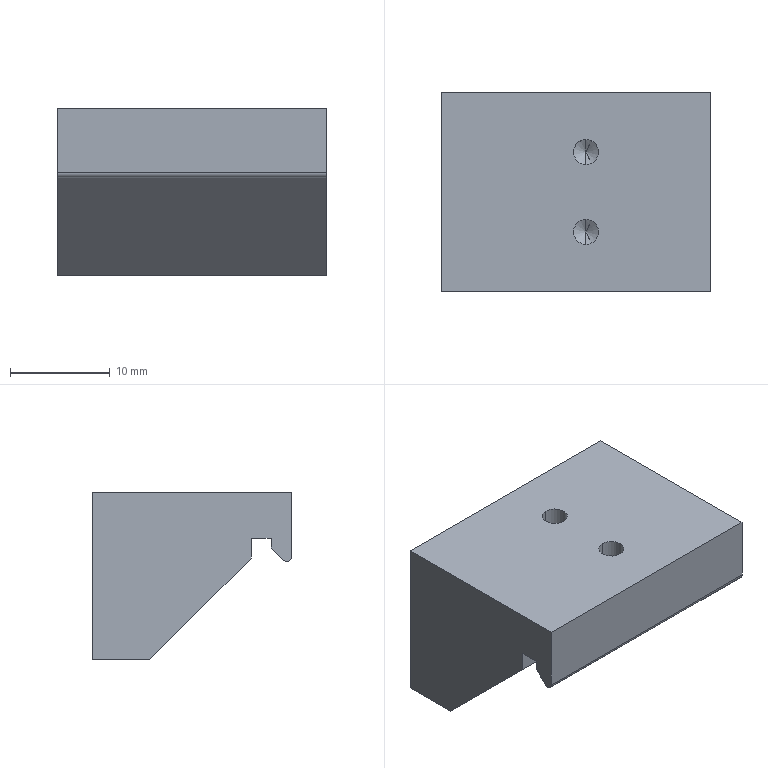NC program | NX | posted with a generic post | part box 27 x 20 x 16.8 mm
Whole program, first 1866 of 2263 lines:
N10 G17 G21 G94 G90
(FLOOR_WALL , TOOL : D10JING)
N12 T09 M6
N14 G54
N16 G17 G0 G90 X-23.5 Y11.997 S9500 M3
N18 G43 Z30. H9
N20 Z3.
N22 G94 G1 Z0. F1250.
N24 X-20.5
N26 X20.5
N28 Y6.998
N30 X-20.5
N32 Y1.999
N34 X20.5
N36 Y-3.001
N38 X-20.5
N40 Y-8.
N42 X20.5
N44 X23.5
N46 Z3.
N48 G0 Z30.
N50 M5
(ZLEVEL_PROFILE , TOOL : D10)
N52 T10 M6
N54 G54
N56 G17 G0 G90 X-11.604 Y-15.1 S9500 M3
N58 G43 Z30. H10
N60 Z1.5
N62 G94 G1 X-14.054 Z1.372 F1000.
N64 X-15.398 Y-14.766 Z1.299
N66 X-16.604 Y-14.084 Z1.226
N68 X-17.584 Y-13.104 Z1.154
N70 X-18.266 Y-11.898 Z1.081
N72 X-18.6 Y-10.554 Z1.009
N74 Y10.554 Z-0.098
N76 X-18.266 Y11.898 Z-0.17
N78 X-17.584 Y13.104 Z-0.243
N80 X-16.604 Y14.084 Z-0.315
N82 X-15.398 Y14.766 Z-0.388
N84 X-14.054 Y15.1 Z-0.461
N86 X-13.5 Z-0.49
N88 X13.5 F2500.
N90 G2 X18.6 Y10. R5.1
N92 G1 Y-10.
N94 G2 X13.5 Y-15.1 R5.1
N96 G1 X-13.5
N98 G2 X-18.6 Y-10. R5.1
N100 G1 Y10.
N102 G2 X-13.5 Y15.1 R5.1
N104 G1 X13.039 Z-0.953
N106 X13.418 Z-0.96
N108 X13.797 Y15.091 Z-0.966
N110 X14.174 Y15.055 Z-0.973
N112 X14.548 Y14.991 Z-0.979
N114 G2 X18.6 Y10. R5.1
N116 G1 Y-10.
N118 G2 X13.5 Y-15.1 R5.1
N120 G1 X-13.5
N122 G2 X-18.6 Y-10. R5.1
N124 G1 Y10.
N126 G2 X-13.5 Y15.1 R5.1
N128 G1 X13.039 Z-1.443
N130 X13.418 Z-1.449
N132 X13.797 Y15.091 Z-1.456
N134 X14.174 Y15.055 Z-1.463
N136 X14.548 Y14.991 Z-1.469
N138 G2 X18.6 Y10. R5.1
N140 G1 Y-10.
N142 G2 X13.5 Y-15.1 R5.1
N144 G1 X-13.5
N146 G2 X-18.6 Y-10. R5.1
N148 G1 Y10.
N150 G2 X-13.5 Y15.1 R5.1
N152 G1 X13.039 Z-1.932
N154 X13.418 Z-1.939
N156 X13.797 Y15.091 Z-1.946
N158 X14.174 Y15.055 Z-1.952
N160 X14.548 Y14.991 Z-1.959
N162 G2 X18.6 Y10. R5.1
N164 G1 Y-10.
N166 G2 X13.5 Y-15.1 R5.1
N168 G1 X-13.5
N170 G2 X-18.6 Y-10. R5.1
N172 G1 Y10.
N174 G2 X-13.5 Y15.1 R5.1
N176 G1 X13.039 Z-2.422
N178 X13.418 Z-2.429
N180 X13.797 Y15.091 Z-2.435
N182 X14.174 Y15.055 Z-2.442
N184 X14.548 Y14.991 Z-2.449
N186 G2 X18.6 Y10. R5.1
N188 G1 Y-10.
N190 G2 X13.5 Y-15.1 R5.1
N192 G1 X-13.5
N194 G2 X-18.6 Y-10. R5.1
N196 G1 Y10.
N198 G2 X-13.5 Y15.1 R5.1
N200 G1 X13.039 Z-2.912
N202 X13.418 Z-2.918
N204 X13.797 Y15.091 Z-2.925
N206 X14.174 Y15.055 Z-2.932
N208 X14.548 Y14.991 Z-2.938
N210 G2 X18.6 Y10. R5.1
N212 G1 Y-10.
N214 G2 X13.5 Y-15.1 R5.1
N216 G1 X-13.5
N218 G2 X-18.6 Y-10. R5.1
N220 G1 Y10.
N222 G2 X-13.5 Y15.1 R5.1
N224 G1 X13.039 Z-3.401
N226 X13.418 Z-3.408
N228 X13.797 Y15.091 Z-3.415
N230 X14.174 Y15.055 Z-3.421
N232 X14.548 Y14.991 Z-3.428
N234 G2 X18.6 Y10. R5.1
N236 G1 Y-10.
N238 G2 X13.5 Y-15.1 R5.1
N240 G1 X-13.5
N242 G2 X-18.6 Y-10. R5.1
N244 G1 Y10.
N246 G2 X-13.5 Y15.1 R5.1
N248 G1 X13.039 Z-3.891
N250 X13.418 Z-3.898
N252 X13.797 Y15.091 Z-3.904
N254 X14.174 Y15.055 Z-3.911
N256 X14.548 Y14.991 Z-3.918
N258 G2 X18.6 Y10. R5.1
N260 G1 Y-10.
N262 G2 X13.5 Y-15.1 R5.1
N264 G1 X-13.5
N266 G2 X-18.6 Y-10. R5.1
N268 G1 Y10.
N270 G2 X-13.5 Y15.1 R5.1
N272 G1 X13.039 Z-4.381
N274 X13.418 Z-4.388
N276 X13.797 Y15.091 Z-4.394
N278 X14.174 Y15.055 Z-4.401
N280 X14.548 Y14.991 Z-4.407
N282 G2 X18.6 Y10. R5.1
N284 G1 Y-10.
N286 G2 X13.5 Y-15.1 R5.1
N288 G1 X-13.5
N290 G2 X-18.6 Y-10. R5.1
N292 G1 Y10.
N294 G2 X-13.5 Y15.1 R5.1
N296 G1 X13.039 Z-4.871
N298 X13.418 Z-4.877
N300 X13.797 Y15.091 Z-4.884
N302 X14.174 Y15.055 Z-4.89
N304 X14.548 Y14.991 Z-4.897
N306 G2 X18.6 Y10. R5.1
N308 G1 Y-10.
N310 G2 X13.5 Y-15.1 R5.1
N312 G1 X-13.5
N314 G2 X-18.6 Y-10. R5.1
N316 G1 Y10.
N318 G2 X-13.5 Y15.1 R5.1
N320 G1 X13.039 Z-5.36
N322 X13.418 Z-5.367
N324 X13.797 Y15.091 Z-5.374
N326 X14.174 Y15.055 Z-5.38
N328 X14.548 Y14.991 Z-5.387
N330 G2 X18.6 Y10. R5.1
N332 G1 Y-10.
N334 G2 X13.5 Y-15.1 R5.1
N336 G1 X-13.5
N338 G2 X-18.6 Y-10. R5.1
N340 G1 Y10.
N342 G2 X-13.5 Y15.1 R5.1
N344 G1 X13.039 Z-5.85
N346 X13.418 Z-5.857
N348 X13.797 Y15.091 Z-5.863
N350 X14.174 Y15.055 Z-5.87
N352 X14.548 Y14.991 Z-5.876
N354 G2 X18.6 Y10. R5.1
N356 G1 Y-10.
N358 G2 X13.5 Y-15.1 R5.1
N360 G1 X-13.5
N362 G2 X-18.6 Y-10. R5.1
N364 G1 Y10.
N366 G2 X-13.5 Y15.1 R5.1
N368 G1 X13.039 Z-6.34
N370 X13.418 Z-6.346
N372 X13.797 Y15.091 Z-6.353
N374 X14.174 Y15.055 Z-6.36
N376 X14.548 Y14.991 Z-6.366
N378 G2 X18.6 Y10. R5.1
N380 G1 Y-10.
N382 G2 X13.5 Y-15.1 R5.1
N384 G1 X-13.5
N386 G2 X-18.6 Y-10. R5.1
N388 G1 Y10.
N390 G2 X-13.5 Y15.1 R5.1
N392 G1 X13.039 Z-6.829
N394 X13.418 Z-6.836
N396 X13.797 Y15.091 Z-6.843
N398 X14.174 Y15.055 Z-6.849
N400 X14.548 Y14.991 Z-6.856
N402 G2 X18.6 Y10. R5.1
N404 G1 Y-10.
N406 G2 X13.5 Y-15.1 R5.1
N408 G1 X-13.5
N410 G2 X-18.6 Y-10. R5.1
N412 G1 Y10.
N414 G2 X-13.5 Y15.1 R5.1
N416 G1 X13.039 Z-7.319
N418 X13.418 Z-7.326
N420 X13.797 Y15.091 Z-7.332
N422 X14.174 Y15.055 Z-7.339
N424 X14.548 Y14.991 Z-7.346
N426 G2 X18.6 Y10. R5.1
N428 G1 Y-10.
N430 G2 X13.5 Y-15.1 R5.1
N432 G1 X-13.5
N434 G2 X-18.6 Y-10. R5.1
N436 G1 Y10.
N438 G2 X-13.5 Y15.1 R5.1
N440 G1 X13.039 Z-7.809
N442 X13.418 Z-7.815
N444 X13.797 Y15.091 Z-7.822
N446 X14.174 Y15.055 Z-7.829
N448 X14.548 Y14.991 Z-7.835
N450 G2 X18.6 Y10. R5.1
N452 G1 Y-10.
N454 G2 X13.5 Y-15.1 R5.1
N456 G1 X-13.5
N458 G2 X-18.6 Y-10. R5.1
N460 G1 Y10.
N462 G2 X-13.5 Y15.1 R5.1
N464 G1 X13.039 Z-8.299
N466 X13.418 Z-8.305
N468 X13.797 Y15.091 Z-8.312
N470 X14.174 Y15.055 Z-8.318
N472 X14.548 Y14.991 Z-8.325
N474 G2 X18.6 Y10. R5.1
N476 G1 Y-10.
N478 G2 X13.5 Y-15.1 R5.1
N480 G1 X-13.5
N482 G2 X-18.6 Y-10. R5.1
N484 G1 Y10.
N486 G2 X-13.5 Y15.1 R5.1
N488 G1 X13.039 Z-8.788
N490 X13.418 Z-8.795
N492 X13.797 Y15.091 Z-8.801
N494 X14.174 Y15.055 Z-8.808
N496 X14.548 Y14.991 Z-8.815
N498 G2 X18.6 Y10. R5.1
N500 G1 Y-10.
N502 G2 X13.5 Y-15.1 R5.1
N504 G1 X-13.5
N506 G2 X-18.6 Y-10. R5.1
N508 G1 Y10.
N510 G2 X-13.5 Y15.1 R5.1
N512 G1 X13.039 Z-9.278
N514 X13.418 Z-9.285
N516 X13.797 Y15.091 Z-9.291
N518 X14.174 Y15.055 Z-9.298
N520 X14.548 Y14.991 Z-9.304
N522 G2 X18.6 Y10. R5.1
N524 G1 Y-10.
N526 G2 X13.5 Y-15.1 R5.1
N528 G1 X-13.5
N530 G2 X-18.6 Y-10. R5.1
N532 G1 Y10.
N534 G2 X-13.5 Y15.1 R5.1
N536 G1 X13.039 Z-9.768
N538 X13.418 Z-9.774
N540 X13.797 Y15.091 Z-9.781
N542 X14.174 Y15.055 Z-9.788
N544 X14.548 Y14.991 Z-9.794
N546 G2 X18.6 Y10. R5.1
N548 G1 Y-10.
N550 G2 X13.5 Y-15.1 R5.1
N552 G1 X-13.5
N554 G2 X-18.6 Y-10. R5.1
N556 G1 Y10.
N558 G2 X-13.5 Y15.1 R5.1
N560 G1 X13.039 Z-10.257
N562 X13.418 Z-10.264
N564 X13.797 Y15.091 Z-10.271
N566 X14.174 Y15.055 Z-10.277
N568 X14.548 Y14.991 Z-10.284
N570 G2 X18.6 Y10. R5.1
N572 G1 Y-10.
N574 G2 X13.5 Y-15.1 R5.1
N576 G1 X-13.5
N578 G2 X-18.6 Y-10. R5.1
N580 G1 Y10.
N582 G2 X-13.5 Y15.1 R5.1
N584 G1 X13.039 Z-10.747
N586 X13.418 Z-10.754
N588 X13.797 Y15.091 Z-10.76
N590 X14.174 Y15.055 Z-10.767
N592 X14.548 Y14.991 Z-10.774
N594 G2 X18.6 Y10. R5.1
N596 G1 Y-10.
N598 G2 X13.5 Y-15.1 R5.1
N600 G1 X-13.5
N602 G2 X-18.6 Y-10. R5.1
N604 G1 Y10.
N606 G2 X-13.5 Y15.1 R5.1
N608 G1 X13.039 Z-11.237
N610 X13.418 Z-11.243
N612 X13.797 Y15.091 Z-11.25
N614 X14.174 Y15.055 Z-11.257
N616 X14.548 Y14.991 Z-11.263
N618 G2 X18.6 Y10. R5.1
N620 G1 Y-10.
N622 G2 X13.5 Y-15.1 R5.1
N624 G1 X-13.5
N626 G2 X-18.6 Y-10. R5.1
N628 G1 Y10.
N630 G2 X-13.5 Y15.1 R5.1
N632 G1 X13.039 Z-11.726
N634 X13.418 Z-11.733
N636 X13.797 Y15.091 Z-11.74
N638 X14.174 Y15.055 Z-11.746
N640 X14.548 Y14.991 Z-11.753
N642 G2 X18.6 Y10. R5.1
N644 G1 Y-10.
N646 G2 X13.5 Y-15.1 R5.1
N648 G1 X-13.5
N650 G2 X-18.6 Y-10. R5.1
N652 G1 Y10.
N654 G2 X-13.5 Y15.1 R5.1
N656 G1 X13.039 Z-12.216
N658 X13.418 Z-12.223
N660 X13.797 Y15.091 Z-12.229
N662 X14.174 Y15.055 Z-12.236
N664 X14.548 Y14.991 Z-12.243
N666 G2 X18.6 Y10. R5.1
N668 G1 Y-10.
N670 G2 X13.5 Y-15.1 R5.1
N672 G1 X-13.5
N674 G2 X-18.6 Y-10. R5.1
N676 G1 Y10.
N678 G2 X-13.5 Y15.1 R5.1
N680 G1 X13.039 Z-12.706
N682 X13.418 Z-12.713
N684 X13.797 Y15.091 Z-12.719
N686 X14.174 Y15.055 Z-12.726
N688 X14.548 Y14.991 Z-12.732
N690 G2 X18.6 Y10. R5.1
N692 G1 Y-10.
N694 G2 X13.5 Y-15.1 R5.1
N696 G1 X-13.5
N698 G2 X-18.6 Y-10. R5.1
N700 G1 Y10.
N702 G2 X-13.5 Y15.1 R5.1
N704 G1 X13.039 Z-13.196
N706 X13.418 Z-13.202
N708 X13.797 Y15.091 Z-13.209
N710 X14.174 Y15.055 Z-13.215
N712 X14.548 Y14.991 Z-13.222
N714 G2 X18.6 Y10. R5.1
N716 G1 Y-10.
N718 G2 X13.5 Y-15.1 R5.1
N720 G1 X-13.5
N722 G2 X-18.6 Y-10. R5.1
N724 G1 Y10.
N726 G2 X-13.5 Y15.1 R5.1
N728 G1 X13.039 Z-13.685
N730 X13.418 Z-13.692
N732 X13.797 Y15.091 Z-13.699
N734 X14.174 Y15.055 Z-13.705
N736 X14.548 Y14.991 Z-13.712
N738 G2 X18.6 Y10. R5.1
N740 G1 Y-10.
N742 G2 X13.5 Y-15.1 R5.1
N744 G1 X-13.5
N746 G2 X-18.6 Y-10. R5.1
N748 G1 Y10.
N750 G2 X-13.5 Y15.1 R5.1
N752 G1 X13.039 Z-14.175
N754 X13.418 Z-14.182
N756 X13.797 Y15.091 Z-14.188
N758 X14.174 Y15.055 Z-14.195
N760 X14.548 Y14.991 Z-14.201
N762 G2 X18.6 Y10. R5.1
N764 G1 Y-10.
N766 G2 X13.5 Y-15.1 R5.1
N768 G1 X-13.5
N770 G2 X-18.6 Y-10. R5.1
N772 G1 Y10.
N774 G2 X-13.5 Y15.1 R5.1
N776 G1 X13.039 Z-14.665
N778 X13.418 Z-14.671
N780 X13.797 Y15.091 Z-14.678
N782 X14.174 Y15.055 Z-14.685
N784 X14.548 Y14.991 Z-14.691
N786 G2 X18.6 Y10. R5.1
N788 G1 Y-10.
N790 G2 X13.5 Y-15.1 R5.1
N792 G1 X-13.5
N794 G2 X-18.6 Y-10. R5.1
N796 G1 Y10.
N798 G2 X-13.5 Y15.1 R5.1
N800 G1 X13.039 Z-15.154
N802 X13.418 Z-15.161
N804 X13.797 Y15.091 Z-15.168
N806 X14.174 Y15.055 Z-15.174
N808 X14.548 Y14.991 Z-15.181
N810 G2 X18.6 Y10. R5.1
N812 G1 Y-10.
N814 G2 X13.5 Y-15.1 R5.1
N816 G1 X-13.5
N818 G2 X-18.6 Y-10. R5.1
N820 G1 Y10.
N822 G2 X-13.5 Y15.1 R5.1
N824 G1 X13.039 Z-15.644
N826 X13.418 Z-15.651
N828 X13.797 Y15.091 Z-15.657
N830 X14.174 Y15.055 Z-15.664
N832 X14.548 Y14.991 Z-15.671
N834 G2 X18.6 Y10. R5.1
N836 G1 Y-10.
N838 G2 X13.5 Y-15.1 R5.1
N840 G1 X-13.5
N842 G2 X-18.6 Y-10. R5.1
N844 G1 Y10.
N846 G2 X-13.5 Y15.1 R5.1
N848 G1 X13.039 Z-16.134
N850 X13.418 Z-16.14
N852 X13.797 Y15.091 Z-16.147
N854 X14.174 Y15.055 Z-16.154
N856 X14.548 Y14.991 Z-16.16
N858 G2 X18.6 Y10. R5.1
N860 G1 Y-10.
N862 G2 X13.5 Y-15.1 R5.1
N864 G1 X-13.5
N866 G2 X-18.6 Y-10. R5.1
N868 G1 Y10.
N870 G2 X-13.5 Y15.1 R5.1
N872 G1 X13.039 Z-16.624
N874 X13.418 Z-16.63
N876 X13.797 Y15.091 Z-16.637
N878 X14.174 Y15.055 Z-16.643
N880 X14.548 Y14.991 Z-16.65
N882 G2 X18.6 Y10. R5.1
N884 G1 Y-10.
N886 G2 X13.5 Y-15.1 R5.1
N888 G1 X-13.5
N890 G2 X-18.6 Y-10. R5.1
N892 G1 Y10.
N894 G2 X-13.5 Y15.1 R5.1
N896 G1 X13.5
N898 G2 X14.548 Y14.991 R5.1
N900 G1 Z-15.15
N902 G0 Z30.
(CAVITY_MILL_COPY , TOOL : D6)
N904 T06 M6
N906 G17 G43 G0 G90 X-18.4 Y-9.253 Z30. S9509 H6 M3
N908 Z-8.648
N910 G94 G1 Z-10.148 F1000.
N912 X-17.194 Y-8.914
N914 G3 X-16.495 Y-8.198 R1.
N916 G2 X-16.206 Y-7.448 R3.388 F1500.
N918 X-16.473 Y-6.763 R3.543
N920 G3 X-17.185 Y-6.06 R1.
N922 G1 X-18.4 Y-5.744
N924 Z-8.648
N926 G0 Y-8.951 Z-9.136
N928 G1 Z-10.636 F1000.
N930 X-17.196 Y-8.564
N932 G3 X-16.524 Y-7.823 R1.
N934 G2 X-16.327 Y-7.203 R3.377 F1500.
N936 X-16.528 Y-6.592 R3.1
N938 G3 X-17.202 Y-5.853 R1.
N940 G1 X-18.4 Y-5.472
N942 Z-9.136
N944 G0 Y-8.791 Z-9.624
N946 G1 Z-11.124 F1000.
N948 X-17.187 Y-8.315
N950 G3 X-16.564 Y-7.533 R1.
N952 G2 X-16.424 Y-6.96 R3.276 F1500.
N954 X-16.57 Y-6.359 R3.1
N956 G3 X-17.185 Y-5.57 R1.
N958 G1 X-18.4 Y-5.078
N960 Z-9.624
N962 G0 Y-8.671 Z-10.112
N964 G1 Z-11.612 F1000.
N966 X-17.192 Y-8.211
N968 G3 X-16.56 Y-7.436 R1.
N970 G2 X-16.434 Y-6.93 R3.1 F1500.
N972 X-16.56 Y-6.424 R3.1
N974 G3 X-17.192 Y-5.649 R1.
N976 G1 X-18.4 Y-5.189
N978 Z-10.112
N980 G0 Y-8.671 Z-10.6
N982 G1 Z-12.1 F1000.
N984 X-17.192 Y-8.211
N986 G3 X-16.56 Y-7.436 R1.
N988 G2 X-16.434 Y-6.93 R3.1 F1500.
N990 X-16.56 Y-6.424 R3.1
N992 G3 X-17.192 Y-5.649 R1.
N994 G1 X-18.4 Y-5.189
N996 Z-10.6
N998 G0 Z30.
N1000 X18.4 Y-5.728
N1002 Z-8.648
N1004 G1 Z-10.148 F1000.
N1006 X17.197 Y-6.036
N1008 G3 X16.482 Y-6.736 R1.
N1010 G2 X16.196 Y-7.43 R3.193 F1500.
N1012 X16.483 Y-8.133 R3.235
N1014 G3 X17.196 Y-8.834 R1.
N1016 G1 X18.4 Y-9.146
N1018 Z-8.648
N1020 G0 Y-5.473 Z-9.136
N1022 G1 Z-10.636 F1000.
N1024 X17.202 Y-5.854
N1026 G3 X16.528 Y-6.593 R1.
N1028 G2 X16.326 Y-7.203 R3.1 F1500.
N1030 X16.524 Y-7.821 R3.364
N1032 G3 X17.196 Y-8.562 R1.
N1034 G1 X18.4 Y-8.948
N1036 Z-9.136
N1038 G0 Y-5.189 Z-9.624
N1040 G1 Z-11.124 F1000.
N1042 X17.192 Y-5.649
N1044 G3 X16.56 Y-6.424 R1.
N1046 G2 X16.424 Y-6.96 R3.1 F1500.
N1048 X16.558 Y-7.493 R3.231
N1050 G3 X17.191 Y-8.268 R1.
N1052 G1 X18.4 Y-8.726
N1054 Z-9.624
N1056 G0 Y-5.189 Z-10.112
N1058 G1 Z-11.612 F1000.
N1060 X17.192 Y-5.649
N1062 G3 X16.56 Y-6.424 R1.
N1064 G2 X16.434 Y-6.93 R3.1 F1500.
N1066 X16.56 Y-7.436 R3.1
N1068 G3 X17.192 Y-8.211 R1.
N1070 G1 X18.4 Y-8.671
N1072 Z-10.112
N1074 G0 Y-5.189 Z-10.6
N1076 G1 Z-12.1 F1000.
N1078 X17.192 Y-5.649
N1080 G3 X16.56 Y-6.424 R1.
N1082 G2 X16.434 Y-6.93 R3.1 F1500.
N1084 X16.56 Y-7.436 R3.1
N1086 G3 X17.192 Y-8.211 R1.
N1088 G1 X18.4 Y-8.671
N1090 Z-10.6
N1092 G0 Z30.
N1094 M5
(CAVITY_MILL_COPY_COPY , TOOL : D2)
N1096 T02 M6
N1098 G54
N1100 G17 G0 G90 X-15.288 Y-6.21 S9974 M3
N1102 G43 Z30. H2
N1104 Z-8.4
N1106 G94 G1 Z-9.9 F1000.
N1108 G2 X-14.659 Y-6.738 R1.
N1110 G1 X-14.643 Y-6.769
N1112 G2 X-14.649 Y-8.137 R1.56
N1114 G3 X-14.501 Y-8.758 R0.5
N1116 G2 X-13.5 Y-8.089 R1.135
N1118 G1 X13.5
N1120 G2 X14.502 Y-8.76 R1.135
N1122 G3 X14.648 Y-8.134 R0.5
N1124 G2 X14.645 Y-6.734 R1.56
N1126 G3 X14.5 Y-6.113 R0.5
N1128 G2 X13.5 Y-6.771 R1.121
N1130 G1 X-13.5
N1132 G2 X-14.514 Y-6.082 R1.121
N1134 G3 X-14.659 Y-6.738 R0.501
N1136 G2 X-14.732 Y-7.735 R1.
N1138 G1 X-15.284 Y-8.546
N1140 Z-8.4
N1142 G0 X-15.256 Y-6.137 Z-8.6
N1144 G1 Z-10.1
N1146 G2 X-14.761 Y-6.765 R1.
N1148 G1 X-14.744 Y-6.816
N1150 X-14.707 Y-6.925
N1152 X-14.685 Y-6.999
N1154 G2 X-14.73 Y-8.025 R1.56
N1156 G3 X-14.535 Y-8.632 R0.5
N1158 G2 X-13.5 Y-7.889 R1.121
N1160 G1 X13.5
N1162 G2 X14.532 Y-8.625 R1.121
N1164 G3 X14.724 Y-8.017 R0.5
N1166 G2 X14.724 Y-6.843 R1.56
N1168 G3 X14.532 Y-6.235 R0.5
N1170 G2 X13.5 Y-6.971 R1.121
N1172 G1 X-13.5
N1174 G2 X-14.54 Y-6.213 R1.121
N1176 G3 X-14.761 Y-6.765 R0.5
N1178 G2 X-15.025 Y-7.729 R1.
N1180 G1 X-15.354 Y-8.055
N1182 Z-8.6
N1184 G0 X-15.241 Y-6.106 Z-8.8
N1186 G1 Z-10.3
N1188 G2 X-14.795 Y-6.771 R1.
N1190 G1 X-14.774 Y-6.85
N1192 G2 X-14.767 Y-7.878 R1.56
N1194 G3 X-14.548 Y-8.471 R0.5
N1196 G2 X-13.5 Y-7.689 R1.121
N1198 G1 X13.5
N1200 G2 X14.55 Y-8.478 R1.121
N1202 G3 X14.772 Y-7.882 R0.5
N1204 G2 X14.775 Y-6.848 R1.56
N1206 G3 X14.553 Y-6.247 R0.5
N1208 G2 X13.5 Y-7.03 R1.1
N1210 G1 X-13.5
N1212 G2 X-14.553 Y-6.249 R1.1
N1214 G3 X-14.795 Y-6.771 R0.5
N1216 G2 X-15.133 Y-7.712 R1.
N1218 G1 X-15.389 Y-7.929
N1220 Z-8.8
N1222 G0 X-15.308 Y-6.146 Z-9.
N1224 G1 Z-10.5
N1226 G2 X-14.815 Y-6.776 R1.
N1228 G1 X-14.808 Y-6.801
N1230 G2 X-14.805 Y-7.729 R1.56
N1232 G3 X-14.561 Y-8.317 R0.5
N1234 G2 X-13.5 Y-7.489 R1.121
N1236 G1 X13.5
N1238 G2 X14.561 Y-8.317 R1.121
N1240 G3 X14.805 Y-7.729 R0.5
N1242 G2 X14.808 Y-6.801 R1.56
N1244 G3 X14.564 Y-6.209 R0.5
N1246 G2 X13.5 Y-7.03 R1.1
N1248 G1 X-13.5
N1250 G2 X-14.564 Y-6.209 R1.1
N1252 G3 X-14.815 Y-6.776 R0.5
N1254 G2 X-15.083 Y-7.739 R1.
N1256 G1 X-15.411 Y-8.061
N1258 Z-9.
N1260 G0 X-15.344 Y-6.14 Z-9.2
N1262 G1 Z-10.7
N1264 G2 X-14.831 Y-6.78 R1.
N1266 X-14.834 Y-7.575 R1.56
N1268 G3 X-14.571 Y-8.154 R0.5
N1270 G2 X-13.5 Y-7.289 R1.121
N1272 G1 X13.5
N1274 G2 X14.571 Y-8.154 R1.121
N1276 G3 X14.834 Y-7.575 R0.5
N1278 G2 X14.837 Y-6.755 R1.56
N1280 G3 X14.573 Y-6.171 R0.5
N1282 G2 X13.5 Y-7.03 R1.1
N1284 G1 X-13.5
N1286 G2 X-14.573 Y-6.171 R1.1
N1288 G3 X-14.831 Y-6.78 R0.501
N1290 G2 X-15.098 Y-7.744 R1.
N1292 G1 X-15.399 Y-8.04
N1294 Z-9.2
N1296 G0 X-15.357 Y-6.087 Z-9.4
N1298 G1 Z-10.9
N1300 G2 X-14.849 Y-6.784 R1.
N1302 X-14.865 Y-7.429 R1.56
N1304 G3 X-14.58 Y-8.002 R0.5
N1306 G2 X-13.5 Y-7.089 R1.127
N1308 G1 X13.5
N1310 G2 X14.58 Y-8.005 R1.13
N1312 G3 X14.865 Y-7.431 R0.5
N1314 G2 X14.866 Y-6.707 R1.56
N1316 G3 X14.581 Y-6.133 R0.5
N1318 G2 X13.5 Y-7.03 R1.1
N1320 G1 X-13.5
N1322 G2 X-14.581 Y-6.133 R1.1
N1324 G3 X-14.866 Y-6.707 R0.5
N1326 G1 X-14.849 Y-6.784
N1328 G2 X-15.182 Y-7.727 R1.
N1330 G1 X-15.411 Y-7.923
N1332 Z-9.4
N1334 G0 Z30.
N1336 X15.2 Y-5.316
N1338 Z-9.6
N1340 G1 Z-11.1
N1342 G3 X14.588 Y-6.094 R1.
N1344 G2 X13.886 Y-6.96 R1.1
N1346 X14.587 Y-7.853 R1.153
N1348 G3 X15.2 Y-8.63 R1.
N1350 G1 Z-9.6
N1352 G0 Y-5.294 Z-9.8
N1354 G1 Z-11.3
N1356 G3 X14.59 Y-6.081 R1.
N1358 G2 X13.958 Y-6.93 R1.1
N1360 X14.59 Y-7.779 R1.1
N1362 G3 X15.2 Y-8.566 R1.
N1364 G1 Z-9.8
N1366 G0 Y-5.294 Z-10.
N1368 G1 Z-11.5
N1370 G3 X14.59 Y-6.081 R1.
N1372 G2 X13.958 Y-6.93 R1.1
N1374 X14.59 Y-7.779 R1.1
N1376 G3 X15.2 Y-8.566 R1.
N1378 G1 Z-10.
N1380 G0 Y-5.294 Z-10.2
N1382 G1 Z-11.7
N1384 G3 X14.59 Y-6.081 R1.
N1386 G2 X13.958 Y-6.93 R1.1
N1388 X14.59 Y-7.779 R1.1
N1390 G3 X15.2 Y-8.566 R1.
N1392 G1 Z-10.2
N1394 G0 Y-5.294 Z-10.4
N1396 G1 Z-11.9
N1398 G3 X14.59 Y-6.081 R1.
N1400 G2 X13.958 Y-6.93 R1.1
N1402 X14.59 Y-7.779 R1.1
N1404 G3 X15.2 Y-8.566 R1.
N1406 G1 Z-10.4
N1408 G0 Y-5.294 Z-10.6
N1410 G1 Z-12.1
N1412 G3 X14.59 Y-6.081 R1.
N1414 G2 X13.958 Y-6.93 R1.1
N1416 X14.59 Y-7.779 R1.1
N1418 G3 X15.2 Y-8.566 R1.
N1420 G1 Z-10.6
N1422 G0 Z30.
N1424 X-15.2 Y-8.622
N1426 Z-9.6
N1428 G1 Z-11.1
N1430 G3 X-14.587 Y-7.846 R1.
N1432 G2 X-13.886 Y-6.96 R1.139
N1434 X-14.588 Y-6.094 R1.1
N1436 G3 X-15.2 Y-5.316 R1.
N1438 G1 Z-9.6
N1440 G0 Y-8.566 Z-9.8
N1442 G1 Z-11.3
N1444 G3 X-14.59 Y-7.779 R1.
N1446 G2 X-13.958 Y-6.93 R1.1
N1448 X-14.59 Y-6.081 R1.1
N1450 G3 X-15.2 Y-5.294 R1.
N1452 G1 Z-9.8
N1454 G0 Y-8.566 Z-10.
N1456 G1 Z-11.5
N1458 G3 X-14.59 Y-7.779 R1.
N1460 G2 X-13.958 Y-6.93 R1.1
N1462 X-14.59 Y-6.081 R1.1
N1464 G3 X-15.2 Y-5.294 R1.
N1466 G1 Z-10.
N1468 G0 Y-8.566 Z-10.2
N1470 G1 Z-11.7
N1472 G3 X-14.59 Y-7.779 R1.
N1474 G2 X-13.958 Y-6.93 R1.1
N1476 X-14.59 Y-6.081 R1.1
N1478 G3 X-15.2 Y-5.294 R1.
N1480 G1 Z-10.2
N1482 G0 Y-8.566 Z-10.4
N1484 G1 Z-11.9
N1486 G3 X-14.59 Y-7.779 R1.
N1488 G2 X-13.958 Y-6.93 R1.1
N1490 X-14.59 Y-6.081 R1.1
N1492 G3 X-15.2 Y-5.294 R1.
N1494 G1 Z-10.4
N1496 G0 Y-8.566 Z-10.6
N1498 G1 Z-12.1
N1500 G3 X-14.59 Y-7.779 R1.
N1502 G2 X-13.958 Y-6.93 R1.1
N1504 X-14.59 Y-6.081 R1.1
N1506 G3 X-15.2 Y-5.294 R1.
N1508 G1 Z-10.6
N1510 G0 Z30.
(PLANAR_PROFILE , TOOL : D2)
N1512 X17.5 Y-6.93 S9500
N1514 Z-7.35
N1516 G1 Z-10.35 F1250.
N1518 X13.5
N1520 X-13.5
N1522 X-17.5
N1524 Z-7.35
N1526 G0 Z-7.5
N1528 G1 Z-10.5
N1530 X-13.5
N1532 X13.5
N1534 X17.5
N1536 Z-7.5
N1538 G0 Z-7.65
N1540 G1 Z-10.65
N1542 X13.5
N1544 X-13.5
N1546 X-17.5
N1548 Z-7.65
N1550 G0 Z-7.8
N1552 G1 Z-10.8
N1554 X-13.5
N1556 X13.5
N1558 X17.5
N1560 Z-7.8
N1562 G0 Z-7.95
N1564 G1 Z-10.95
N1566 X13.5
N1568 X-13.5
N1570 X-17.5
N1572 Z-7.95
N1574 G0 Z-8.1
N1576 G1 Z-11.1
N1578 X-13.5
N1580 X13.5
N1582 X17.5
N1584 Z-8.1
N1586 G0 Z-8.25
N1588 G1 Z-11.25
N1590 X13.5
N1592 X-13.5
N1594 X-17.5
N1596 Z-8.25
N1598 G0 Z-8.4
N1600 G1 Z-11.4
N1602 X-13.5
N1604 X13.5
N1606 X17.5
N1608 Z-8.4
N1610 G0 Z-8.55
N1612 G1 Z-11.55
N1614 X13.5
N1616 X-13.5
N1618 X-17.5
N1620 Z-8.55
N1622 G0 Z-8.7
N1624 G1 Z-11.7
N1626 X-13.5
N1628 X13.5
N1630 X17.5
N1632 Z-8.7
N1634 G0 Z-8.85
N1636 G1 Z-11.85
N1638 X13.5
N1640 X-13.5
N1642 X-17.5
N1644 Z-8.85
N1646 G0 Z-9.
N1648 G1 Z-12.
N1650 X-13.5
N1652 X13.5
N1654 X17.5
N1656 Z-9.
N1658 G0 Z-9.15
N1660 G1 Z-12.15
N1662 X13.5
N1664 X-13.5
N1666 X-17.5
N1668 Z-9.15
N1670 G0 Z-9.2
N1672 G1 Z-12.2
N1674 X-13.5
N1676 X13.5
N1678 X17.5
N1680 Z-9.2
N1682 G0 Z30.
N1684 M5
(ZLEVEL_PROFILE_1 , TOOL : D2R0.5)
N1686 T05 M6
N1688 G54
N1690 G17 G0 G90 X14.797 Y3.149 S9500 M3
N1692 G43 Z30. H5
N1694 Z2.943
N1696 G94 G1 Z-0.057 F1000.
N1698 X14.648 Y3.407
N1700 G3 X14.475 Y3.507 R0.2
N1702 G1 X-14.475 F2500.
N1704 Y3.478 Z-0.085
N1706 Y3.45 Z-0.113
N1708 X14.475
N1710 X14.476 Y3.421 Z-0.141
N1712 Y3.394 Z-0.17
N1714 X13.5 Y3.393
N1716 X-13.5
N1718 X-14.476 Y3.394
N1720 Y3.365 Z-0.198
N1722 Y3.337 Z-0.226
N1724 X-13.5
N1726 X13.5
N1728 X14.476
N1730 X14.477 Y3.308 Z-0.255
N1732 Y3.281 Z-0.283
N1734 X13.5 Y3.28
N1736 X-13.5
N1738 X-14.477 Y3.281
N1740 Y3.252 Z-0.311
N1742 Y3.224 Z-0.339
N1744 X-13.5 Y3.223
N1746 X13.5
N1748 X14.478 Y3.224
N1750 Y3.195 Z-0.368
N1752 Y3.167 Z-0.396
N1754 X13.5
N1756 X-13.5
N1758 X-14.478
N1760 Y3.139 Z-0.424
N1762 Y3.111 Z-0.453
N1764 X-13.5 Y3.11
N1766 X13.5
N1768 X14.478 Y3.111
N1770 X14.479 Y3.082 Z-0.481
N1772 Y3.054 Z-0.509
N1774 X13.5
N1776 X-13.5
N1778 X-14.479
N1780 Y3.025 Z-0.537
N1782 Y2.998 Z-0.566
N1784 X-13.5 Y2.997
N1786 X13.5
N1788 X14.479 Y2.998
N1790 X14.48 Y2.969 Z-0.594
N1792 Y2.941 Z-0.622
N1794 X13.5
N1796 X-13.5
N1798 X-14.48
N1800 Y2.912 Z-0.651
N1802 Y2.885 Z-0.679
N1804 X-13.5 Y2.884
N1806 X13.5
N1808 X14.48 Y2.885
N1810 X14.481 Y2.856 Z-0.707
N1812 Y2.828 Z-0.735
N1814 X13.5
N1816 X-13.5
N1818 X-14.481
N1820 Y2.799 Z-0.764
N1822 Y2.771 Z-0.792
N1824 X-13.5
N1826 X13.5
N1828 X14.481
N1830 X14.482 Y2.743 Z-0.82
N1832 Y2.715 Z-0.849
N1834 X13.5 Y2.714
N1836 X-13.5
N1838 X-14.482 Y2.715
N1840 Y2.686 Z-0.877
N1842 Y2.658 Z-0.905
N1844 X-13.5
N1846 X13.5
N1848 X14.482
N1850 X14.483 Y2.63 Z-0.933
N1852 Y2.602 Z-0.962
N1854 X13.5 Y2.601
N1856 X-13.5
N1858 X-14.483 Y2.602
N1860 Y2.573 Z-0.99
N1862 Y2.545 Z-1.018
N1864 X-13.5
N1866 X13.5
N1868 X14.483
N1870 X14.484 Y2.516 Z-1.047
N1872 Y2.488 Z-1.075
N1874 X13.5
N1876 X-13.5
N1878 X-14.484
N1880 Y2.46 Z-1.103
N1882 Y2.432 Z-1.131
N1884 X-13.5
N1886 X13.5
N1888 X14.485
N1890 Y2.403 Z-1.16
N1892 Y2.375 Z-1.188
N1894 X13.5
N1896 X-13.5
N1898 X-14.485
N1900 Y2.347 Z-1.216
N1902 Y2.319 Z-1.245
N1904 X-13.5 Y2.318
N1906 X13.5
N1908 X14.485 Y2.319
N1910 X14.486 Y2.29 Z-1.273
N1912 Y2.262 Z-1.301
N1914 X13.5
N1916 X-13.5
N1918 X-14.486
N1920 Y2.234 Z-1.329
N1922 Y2.206 Z-1.358
N1924 X-13.5 Y2.205
N1926 X13.5
N1928 X14.486 Y2.206
N1930 X14.487 Y2.177 Z-1.386
N1932 Y2.149 Z-1.414
N1934 X13.5
N1936 X-13.5
N1938 X-14.487
N1940 Y2.12 Z-1.442
N1942 Y2.092 Z-1.471
N1944 X-13.5
N1946 X13.5
N1948 X14.487
N1950 X14.488 Y2.064 Z-1.499
N1952 Y2.036 Z-1.527
N1954 X13.5
N1956 X-13.5
N1958 X-14.488
N1960 Y2.007 Z-1.556
N1962 Y1.979 Z-1.584
N1964 X-13.5
N1966 X13.5
N1968 X14.488
N1970 Y1.951 Z-1.612
N1972 Y1.923 Z-1.64
N1974 X13.5 Y1.922
N1976 X-13.5
N1978 X-14.488 Y1.923
N1980 X-14.489 Y1.894 Z-1.669
N1982 Y1.866 Z-1.697
N1984 X-13.5
N1986 X13.5
N1988 X14.489
N1990 Y1.838 Z-1.725
N1992 Y1.81 Z-1.754
N1994 X13.5 Y1.809
N1996 X-13.5
N1998 X-14.489 Y1.81
N2000 Y1.781 Z-1.782
N2002 Y1.753 Z-1.81
N2004 X-13.5
N2006 X13.5
N2008 X14.489
N2010 X14.49 Y1.724 Z-1.838
N2012 Y1.696 Z-1.867
N2014 X13.5
N2016 X-13.5
N2018 X-14.49
N2020 Y1.668 Z-1.895
N2022 Y1.64 Z-1.923
N2024 X-13.5
N2026 X13.5
N2028 X14.49
N2030 Y1.611 Z-1.952
N2032 Y1.583 Z-1.98
N2034 X13.5
N2036 X-13.5
N2038 X-14.49
N2040 X-14.491 Y1.555 Z-2.008
N2042 Y1.527 Z-2.036
N2044 X-13.5 Y1.526
N2046 X13.5
N2048 X14.491 Y1.527
N2050 Y1.498 Z-2.065
N2052 Y1.47 Z-2.093
N2054 X13.5
N2056 X-13.5
N2058 X-14.491
N2060 Y1.442 Z-2.121
N2062 Y1.413 Z-2.15
N2064 X-13.5
N2066 X13.5
N2068 X14.491
N2070 X14.492 Y1.385 Z-2.178
N2072 Y1.357 Z-2.206
N2074 X13.5
N2076 X-13.5
N2078 X-14.492
N2080 Y1.328 Z-2.234
N2082 Y1.3 Z-2.263
N2084 X-13.5
N2086 X13.5
N2088 X14.492
N2090 Y1.272 Z-2.291
N2092 Y1.244 Z-2.319
N2094 X13.5
N2096 X-13.5
N2098 X-14.492
N2100 X-14.493 Y1.215 Z-2.348
N2102 Y1.187 Z-2.376
N2104 X-13.5
N2106 X13.5
N2108 X14.493
N2110 Y1.159 Z-2.404
N2112 Y1.131 Z-2.432
N2114 X13.5 Y1.13
N2116 X-13.5
N2118 X-14.493 Y1.131
N2120 Y1.102 Z-2.461
N2122 Y1.074 Z-2.489
N2124 X-13.5
N2126 X13.5
N2128 X14.493
N2130 X14.494 Y1.046 Z-2.517
N2132 Y1.017 Z-2.546
N2134 X13.5
N2136 X-13.5
N2138 X-14.494
N2140 Y0.989 Z-2.574
N2142 Y0.961 Z-2.602
N2144 X-13.5
N2146 X13.5
N2148 X14.494
N2150 Y0.932 Z-2.63
N2152 Y0.904 Z-2.659
N2154 X13.5
N2156 X-13.5
N2158 X-14.494
N2160 X-14.495 Y0.876 Z-2.687
N2162 Y0.848 Z-2.715
N2164 X-13.5
N2166 X13.5
N2168 X14.495
N2170 Y0.819 Z-2.744
N2172 Y0.791 Z-2.772
N2174 X13.5
N2176 X-13.5
N2178 X-14.495
N2180 Y0.763 Z-2.8
N2182 Y0.735 Z-2.828
N2184 X-13.5 Y0.734
N2186 X13.5
N2188 X14.495 Y0.735
N2190 Y0.706 Z-2.857
N2192 Y0.678 Z-2.885
N2194 X13.5
N2196 X-13.5
N2198 X-14.495
N2200 Y0.65 Z-2.913
N2202 Y0.621 Z-2.942
N2204 X-13.5
N2206 X13.5
N2208 X14.495
N2210 X14.496 Y0.593 Z-2.97
N2212 Y0.565 Z-2.998
N2214 X13.5
N2216 X-13.5
N2218 X-14.496
N2220 Y0.536 Z-3.026
N2222 Y0.508 Z-3.055
N2224 X-13.5
N2226 X13.5
N2228 X14.496
N2230 Y0.48 Z-3.083
N2232 Y0.452 Z-3.111
N2234 X13.5
N2236 X-13.5
N2238 X-14.496
N2240 Y0.423 Z-3.14
N2242 Y0.395 Z-3.168
N2244 X-13.5
N2246 X13.5
N2248 X14.496
N2250 Y0.367 Z-3.196
N2252 Y0.339 Z-3.224
N2254 X13.5 Y0.338
N2256 X-13.5
N2258 X-14.496 Y0.339
N2260 Y0.31 Z-3.253
N2262 Y0.282 Z-3.281
N2264 X-13.5
N2266 X13.5
N2268 X14.496
N2270 Y0.254 Z-3.309
N2272 Y0.225 Z-3.338
N2274 X13.5
N2276 X-13.5
N2278 X-14.496
N2280 X-14.497 Y0.197 Z-3.366
N2282 Y0.169 Z-3.394
N2284 X-13.5
N2286 X13.5
N2288 X14.497
N2290 Y0.14 Z-3.422
N2292 Y0.112 Z-3.451
N2294 X13.5
N2296 X-13.5
N2298 X-14.497
N2300 Y0.084 Z-3.479
N2302 Y0.056 Z-3.507
N2304 X-13.5
N2306 X13.5
N2308 X14.497
N2310 Y0.027 Z-3.536
N2312 Y-0.001 Z-3.564
N2314 X13.5
N2316 X-13.5
N2318 X-14.497
N2320 Y-0.029 Z-3.592
N2322 Y-0.057 Z-3.62
N2324 X-13.5
N2326 X13.5
N2328 X14.497
N2330 Y-0.086 Z-3.649
N2332 Y-0.114 Z-3.677
N2334 X13.5
N2336 X-13.5
N2338 X-14.497
N2340 X-14.498 Y-0.142 Z-3.705
N2342 Y-0.171 Z-3.734
N2344 X-13.5
N2346 X13.5
N2348 X14.498
N2350 Y-0.199 Z-3.762
N2352 Y-0.227 Z-3.79
N2354 X13.5
N2356 X-13.5
N2358 X-14.498
N2360 Y-0.255 Z-3.818
N2362 Y-0.284 Z-3.847
N2364 X-13.5
N2366 X13.5
N2368 X14.498
N2370 Y-0.312 Z-3.875
N2372 Y-0.34 Z-3.903
N2374 X13.5
N2376 X-13.5
N2378 X-14.498
N2380 Y-0.369 Z-3.932
N2382 Y-0.397 Z-3.96
N2384 X-13.5
N2386 X13.5
N2388 X14.498
N2390 Y-0.425 Z-3.988
N2392 Y-0.453 Z-4.016
N2394 X13.5
N2396 X-13.5
N2398 X-14.498
N2400 Y-0.482 Z-4.045
N2402 Y-0.51 Z-4.073
N2404 X-13.5
N2406 X13.5
N2408 X14.498
N2410 Y-0.538 Z-4.101
N2412 Y-0.567 Z-4.13
N2414 X13.5
N2416 X-13.5
N2418 X-14.498
N2420 Y-0.595 Z-4.158
N2422 Y-0.623 Z-4.186
N2424 X-13.5
N2426 X13.5
N2428 X14.498
N2430 Y-0.651 Z-4.214
N2432 Y-0.68 Z-4.243
N2434 X13.5
N2436 X-13.5
N2438 X-14.498
N2440 Y-0.708 Z-4.271
N2442 Y-0.736 Z-4.299
N2444 X-13.5
N2446 X13.5
N2448 X14.499
N2450 Y-0.765 Z-4.327
N2452 Y-0.793 Z-4.356
N2454 X13.5
N2456 X-13.5
N2458 X-14.498
N2460 Y-0.821 Z-4.384
N2462 X-14.499 Y-0.849 Z-4.412
N2464 X-13.5
N2466 X13.5
N2468 X14.499
N2470 Y-0.878 Z-4.441
N2472 Y-0.906 Z-4.469
N2474 X13.5
N2476 X-13.5
N2478 X-14.499
N2480 Y-0.934 Z-4.497
N2482 Y-0.963 Z-4.525
N2484 X-13.5
N2486 X13.5
N2488 X14.499
N2490 Y-0.991 Z-4.554
N2492 Y-1.019 Z-4.582
N2494 X13.5
N2496 X-13.5
N2498 X-14.499
N2500 Y-1.047 Z-4.61
N2502 Y-1.076 Z-4.639
N2504 X-13.5
N2506 X13.5
N2508 X14.499
N2510 Y-1.104 Z-4.667
N2512 Y-1.132 Z-4.695
N2514 X13.5
N2516 X-13.5
N2518 X-14.499
N2520 Y-1.161 Z-4.723
N2522 Y-1.189 Z-4.752
N2524 X-13.5
N2526 X13.5
N2528 X14.499
N2530 Y-1.217 Z-4.78
N2532 Y-1.245 Z-4.808
N2534 X13.5
N2536 X-13.5
N2538 X-14.499
N2540 Y-1.274 Z-4.837
N2542 Y-1.302 Z-4.865
N2544 X-13.5
N2546 X13.5
N2548 X14.499
N2550 Y-1.33 Z-4.893
N2552 Y-1.359 Z-4.921
N2554 X13.5
N2556 X-13.5
N2558 X-14.499
N2560 Y-1.387 Z-4.95
N2562 Y-1.415 Z-4.978
N2564 X-13.5
N2566 X13.5
N2568 X14.499
N2570 Y-1.443 Z-5.006
N2572 Y-1.472 Z-5.035
N2574 X13.5
N2576 X-13.5
N2578 X-14.499
N2580 Y-1.5 Z-5.063
N2582 Y-1.528 Z-5.091
N2584 X-13.5
N2586 X13.5
N2588 X14.499
N2590 Y-1.557 Z-5.119
N2592 Y-1.585 Z-5.148
N2594 X13.5
N2596 X-13.5
N2598 X-14.499
N2600 Y-1.613 Z-5.176
N2602 Y-1.641 Z-5.204
N2604 X-13.5
N2606 X13.5
N2608 X14.499
N2610 Y-1.67 Z-5.233
N2612 Y-1.698 Z-5.261
N2614 X13.5
N2616 X-13.5
N2618 X-14.499
N2620 Y-1.726 Z-5.289
N2622 Y-1.754 Z-5.317
N2624 X-13.5 Y-1.755
N2626 X13.5
N2628 X14.499 Y-1.754
N2630 Y-1.783 Z-5.346
N2632 Y-1.811 Z-5.374
N2634 X13.5
N2636 X-13.5
N2638 X-14.499
N2640 Y-1.839 Z-5.402
N2642 Y-1.868 Z-5.431
N2644 X-13.5
N2646 X13.5
N2648 X14.499
N2650 Y-1.896 Z-5.459
N2652 Y-1.924 Z-5.487
N2654 X13.5
N2656 X-13.5
N2658 X-14.499
N2660 Y-1.953 Z-5.515
N2662 Y-1.981 Z-5.544
N2664 X-13.5
N2666 X13.5
N2668 X14.499
N2670 Y-2.009 Z-5.572
N2672 Y-2.037 Z-5.6
N2674 X13.5
N2676 X-13.5
N2678 X-14.499
N2680 Y-2.066 Z-5.629
N2682 Y-2.094 Z-5.657
N2684 X-13.5
N2686 X13.5
N2688 X14.499
N2690 Y-2.122 Z-5.685
N2692 Y-2.15 Z-5.713
N2694 X13.5 Y-2.151
N2696 X-13.5
N2698 X-14.499 Y-2.15
N2700 Y-2.179 Z-5.742
N2702 Y-2.207 Z-5.77
N2704 X-13.5
N2706 X13.5
N2708 X14.499
N2710 Y-2.235 Z-5.798
N2712 Y-2.264 Z-5.827
N2714 X13.5
N2716 X-13.5
N2718 X-14.499
N2720 Y-2.292 Z-5.855
N2722 Y-2.32 Z-5.883
N2724 X-13.5
N2726 X13.5
N2728 X14.499
N2730 Y-2.349 Z-5.911
N2732 Y-2.377 Z-5.94
N2734 X13.5
N2736 X-13.5
N2738 X-14.499
N2740 Y-2.405 Z-5.968
N2742 Y-2.433 Z-5.996
N2744 X-13.5
N2746 X13.5
N2748 X14.499
N2750 Y-2.462 Z-6.025
N2752 Y-2.49 Z-6.053
N2754 X13.5
N2756 X-13.5
N2758 X-14.499
N2760 Y-2.518 Z-6.081
N2762 Y-2.546 Z-6.109
N2764 X-13.5 Y-2.547
N2766 X13.5
N2768 X14.499 Y-2.546
N2770 Y-2.575 Z-6.138
N2772 Y-2.603 Z-6.166
N2774 X13.5
N2776 X-13.5
N2778 X-14.498
N2780 Y-2.631 Z-6.194
N2782 Y-2.66 Z-6.223
N2784 X-13.5
N2786 X13.5
N2788 X14.499
N2790 Y-2.688 Z-6.251
N2792 X14.498 Y-2.716 Z-6.279
N2794 X13.5
N2796 X-13.5
N2798 X-14.498
N2800 Y-2.745 Z-6.307
N2802 Y-2.773 Z-6.336
N2804 X-13.5
N2806 X13.5
N2808 X14.498
N2810 Y-2.801 Z-6.364
N2812 Y-2.829 Z-6.392
N2814 X13.5
N2816 X-13.5
N2818 X-14.498
N2820 Y-2.858 Z-6.421
N2822 Y-2.886 Z-6.449
N2824 X-13.5
N2826 X13.5
N2828 X14.498
N2830 Y-2.914 Z-6.477
N2832 Y-2.942 Z-6.505
N2834 X13.5
N2836 X-13.5
N2838 X-14.498
N2840 Y-2.971 Z-6.534
N2842 Y-2.999 Z-6.562
N2844 X-13.5
N2846 X13.5
N2848 X14.498
N2850 Y-3.027 Z-6.59
N2852 Y-3.056 Z-6.619
N2854 X13.5
N2856 X-13.5
N2858 X-14.498
N2860 Y-3.084 Z-6.647
N2862 Y-3.112 Z-6.675
N2864 X-13.5
N2866 X13.5
N2868 X14.498
N2870 Y-3.14 Z-6.703
N2872 Y-3.169 Z-6.732
N2874 X13.5
N2876 X-13.5
N2878 X-14.498
N2880 Y-3.197 Z-6.76
N2882 Y-3.225 Z-6.788
N2884 X-13.5
N2886 X13.5
N2888 X14.498
N2890 Y-3.254 Z-6.817
N2892 X14.497 Y-3.282 Z-6.845
N2894 X13.5
N2896 X-13.5
N2898 X-14.497
N2900 Y-3.31 Z-6.873
N2902 Y-3.338 Z-6.901
N2904 X-13.5
N2906 X13.5
N2908 X14.497
N2910 Y-3.367 Z-6.93
N2912 Y-3.395 Z-6.958
N2914 X13.5
N2916 X-13.5
N2918 X-14.497
N2920 Y-3.423 Z-6.986
N2922 Y-3.452 Z-7.015
N2924 X-13.5
N2926 X13.5
N2928 X14.497
N2930 Y-3.48 Z-7.043
N2932 Y-3.508 Z-7.071
N2934 X13.5
N2936 X-13.5
N2938 X-14.497
N2940 Y-3.536 Z-7.099
N2942 Y-3.565 Z-7.128
N2944 X-13.5
N2946 X13.5
N2948 X14.497
N2950 X14.496 Y-3.593 Z-7.156
N2952 Y-3.621 Z-7.184
N2954 X13.5
N2956 X-13.5
N2958 X-14.496
N2960 Y-3.65 Z-7.212
N2962 Y-3.678 Z-7.241
N2964 X-13.5
N2966 X13.5
N2968 X14.496
N2970 Y-3.706 Z-7.269
N2972 Y-3.734 Z-7.297
N2974 X13.5
N2976 X-13.5
N2978 X-14.496
N2980 Y-3.763 Z-7.326
N2982 Y-3.791 Z-7.354
N2984 X-13.5
N2986 X13.5
N2988 X14.496
N2990 Y-3.819 Z-7.382
N2992 Y-3.847 Z-7.41
N2994 X13.5 Y-3.848
N2996 X-13.5
N2998 X-14.496 Y-3.847
N3000 Y-3.876 Z-7.439
N3002 Y-3.904 Z-7.467
N3004 X-13.5
N3006 X13.5
N3008 X14.496
N3010 Y-3.932 Z-7.495
N3012 Y-3.961 Z-7.524
N3014 X13.5
N3016 X-13.5
N3018 X-14.495
N3020 Y-3.989 Z-7.552
N3022 Y-4.017 Z-7.58
N3024 X-13.5
N3026 X13.5
N3028 X14.495
N3030 Y-4.046 Z-7.608
N3032 Y-4.074 Z-7.637
N3034 X13.5
N3036 X-13.5
N3038 X-14.495
N3040 Y-4.102 Z-7.665
N3042 Y-4.13 Z-7.693
N3044 X-13.5
N3046 X13.5
N3048 X14.495
N3050 Y-4.159 Z-7.722
N3052 Y-4.187 Z-7.75
N3054 X13.5
N3056 X-13.5
N3058 X-14.495
N3060 Y-4.215 Z-7.778
N3062 Y-4.243 Z-7.806
N3064 X-13.5 Y-4.244
N3066 X13.5
N3068 X14.495 Y-4.243
N3070 X14.494 Y-4.272 Z-7.835
N3072 Y-4.3 Z-7.863
N3074 X13.5
N3076 X-13.5
N3078 X-14.494
N3080 Y-4.328 Z-7.891
N3082 Y-4.357 Z-7.92
N3084 X-13.5
N3086 X13.5
N3088 X14.494
N3090 Y-4.385 Z-7.948
N3092 Y-4.413 Z-7.976
N3094 X13.5
N3096 X-13.5
N3098 X-14.494
N3100 Y-4.442 Z-8.004
N3102 X-14.493 Y-4.47 Z-8.033
N3104 X-13.5
N3106 X13.5
N3108 X14.493
N3110 Y-4.498 Z-8.061
N3112 Y-4.526 Z-8.089
N3114 X13.5
N3116 X-13.5
N3118 X-14.493
N3120 Y-4.555 Z-8.118
N3122 Y-4.583 Z-8.146
N3124 X-13.5
N3126 X13.5
N3128 X14.493
N3130 X14.492 Y-4.611 Z-8.174
N3132 Y-4.639 Z-8.202
N3134 X13.5 Y-4.64
N3136 X-13.5
N3138 X-14.492 Y-4.639
N3140 Y-4.668 Z-8.231
N3142 Y-4.696 Z-8.259
N3144 X-13.5
N3146 X13.5
N3148 X14.492
N3150 Y-4.724 Z-8.287
N3152 Y-4.753 Z-8.316
N3154 X13.5
N3156 X-13.5
N3158 X-14.492
N3160 Y-4.781 Z-8.344
N3162 X-14.491 Y-4.809 Z-8.372
N3164 X-13.5
N3166 X13.5
N3168 X14.491
N3170 Y-4.838 Z-8.4
N3172 Y-4.866 Z-8.429
N3174 X13.5
N3176 X-13.5
N3178 X-14.491
N3180 Y-4.894 Z-8.457
N3182 Y-4.922 Z-8.485
N3184 X-13.5
N3186 X13.5
N3188 X14.491
N3190 X14.49 Y-4.951 Z-8.514
N3192 Y-4.979 Z-8.542
N3194 X13.5
N3196 X-13.5
N3198 X-14.49
N3200 Y-5.007 Z-8.57
N3202 Y-5.035 Z-8.598
N3204 X-13.5 Y-5.036
N3206 X13.5
N3208 X14.49 Y-5.035
N3210 Y-5.064 Z-8.627
N3212 Y-5.092 Z-8.655
N3214 X13.5
N3216 X-13.5
N3218 X-14.49
N3220 X-14.489 Y-5.12 Z-8.683
N3222 Y-5.148 Z-8.712
N3224 X-13.5 Y-5.149
N3226 X13.5
N3228 X14.489 Y-5.148
N3230 Y-5.177 Z-8.74
N3232 Y-5.205 Z-8.768
N3234 X13.5
N3236 X-13.5
N3238 X-14.489
N3240 Y-5.234 Z-8.796
N3242 Y-5.262 Z-8.825
N3244 X-13.5
N3246 X13.5
N3248 X14.489
N3250 X14.488 Y-5.29 Z-8.853
N3252 Y-5.318 Z-8.881
N3254 X13.5
N3256 X-13.5
N3258 X-14.488
N3260 Y-5.347 Z-8.91
N3262 Y-5.375 Z-8.938
N3264 X-13.5
N3266 X13.5
N3268 X14.488
N3270 Y-5.403 Z-8.966
N3272 Y-5.431 Z-8.994
N3274 X13.5 Y-5.432
N3276 X-13.5
N3278 X-14.487 Y-5.431
N3280 Y-5.46 Z-9.023
N3282 Y-5.488 Z-9.051
N3284 X-13.5
N3286 X13.5
N3288 X14.487
N3290 Y-5.516 Z-9.079
N3292 Y-5.544 Z-9.108
N3294 X13.5 Y-5.545
N3296 X-13.5
N3298 X-14.486 Y-5.544
N3300 Y-5.573 Z-9.136
N3302 Y-5.601 Z-9.164
N3304 X-13.5
N3306 X13.5
N3308 X14.486
N3310 Y-5.629 Z-9.192
N3312 Y-5.657 Z-9.221
N3314 X13.5 Y-5.658
N3316 X-13.5
N3318 X-14.486 Y-5.657
N3320 X-14.485 Y-5.686 Z-9.249
N3322 Y-5.714 Z-9.277
N3324 X-13.5
N3326 X13.5
N3328 X14.485
N3330 Y-5.743 Z-9.306
N3332 Y-5.771 Z-9.334
N3334 X13.5
N3336 X-13.5
N3338 X-14.485
N3340 X-14.484 Y-5.799 Z-9.362
N3342 Y-5.827 Z-9.39
N3344 X-13.5
N3346 X13.5
N3348 X14.484
N3350 Y-5.856 Z-9.419
N3352 Y-5.884 Z-9.447
N3354 X13.5
N3356 X-13.5
N3358 X-14.484
N3360 X-14.483 Y-5.912 Z-9.475
N3362 Y-5.94 Z-9.504
N3364 X-13.5 Y-5.941
N3366 X13.5
N3368 X14.483 Y-5.94
N3370 Y-5.969 Z-9.532
N3372 Y-5.997 Z-9.56
N3374 X13.5
N3376 X-13.5
N3378 X-14.483
N3380 X-14.482 Y-6.025 Z-9.588
N3382 Y-6.053 Z-9.617
N3384 X-13.5 Y-6.054
N3386 X13.5
N3388 X14.482 Y-6.053
N3390 Y-6.082 Z-9.645
N3392 Y-6.11 Z-9.673
N3394 X13.5
N3396 X-13.5
N3398 X-14.482
N3400 X-14.481 Y-6.139 Z-9.702
N3402 Y-6.166 Z-9.73
N3404 X-13.5 Y-6.167
N3406 X13.5
N3408 X14.481 Y-6.166
N3410 Y-6.195 Z-9.758
N3412 Y-6.223 Z-9.786
N3414 X13.5
N3416 X-13.5
N3418 X-14.481
N3420 X-14.48 Y-6.252 Z-9.815
N3422 Y-6.28 Z-9.843
N3424 X-13.5
N3426 X13.5
N3428 X14.48
N3430 Y-6.308 Z-9.871
N3432 Y-6.336 Z-9.899
N3434 X13.5 Y-6.337
N3436 X-13.5
N3438 X-14.48 Y-6.336
N3440 X-14.479 Y-6.365 Z-9.928
N3442 Y-6.393 Z-9.956
N3444 X-13.5
N3446 X13.5
N3448 X14.479
N3450 Y-6.421 Z-9.984
N3452 Y-6.449 Z-10.013
N3454 X13.5 Y-6.45
N3456 X-13.5
N3458 X-14.479 Y-6.449
N3460 X-14.478 Y-6.478 Z-10.041
N3462 Y-6.506 Z-10.069
N3464 X-13.5
N3466 X13.5
N3468 X14.478
N3470 Y-6.535 Z-10.097
N3472 Y-6.562 Z-10.126
N3474 X13.5 Y-6.563
N3476 X-13.5
N3478 X-14.478 Y-6.562
N3480 X-14.477 Y-6.591 Z-10.154
N3482 Y-6.619 Z-10.182
N3484 X-13.5
N3486 X13.5
N3488 X14.477
N3490 Y-6.648 Z-10.211
N3492 Y-6.675 Z-10.239
N3494 X13.5 Y-6.676
N3496 X-13.5
N3498 X-14.477 Y-6.675
N3500 X-14.476 Y-6.704 Z-10.267
N3502 Y-6.732 Z-10.295
N3504 X-13.5 Y-6.733
N3506 X13.5
N3508 X14.476 Y-6.732
N3510 Y-6.761 Z-10.324
N3512 Y-6.789 Z-10.352
N3514 X-14.476
N3516 X-14.475 Y-6.817 Z-10.38
N3518 Y-6.845 Z-10.409
N3520 X14.475
N3522 Y-6.874 Z-10.437
N3524 Y-6.902 Z-10.465
N3526 X-14.475
N3528 X-14.474 Y-6.931 Z-10.493
N3530 Y-6.958 Z-10.522
N3532 X14.474
N3534 Y-6.981 Z-10.544
N3536 Y-7.003 Z-10.566
N3538 X-14.474
N3540 Y-7.026 Z-10.589
N3542 X-14.473 Y-7.047 Z-10.611
N3544 X14.473
N3546 Y-7.07 Z-10.633
N3548 Y-7.092 Z-10.655
N3550 X-14.473
N3552 Y-7.115 Z-10.678
N3554 Y-7.136 Z-10.7
N3556 X14.473
N3558 G2 X14.646 Y-7.236 R0.2
N3560 G1 X14.791 Y-7.488
N3562 Z-7.7
N3564 G0 Z30.
(ZLEVEL_PROFILE_1_COPY , TOOL : D2R0.5)
N3566 X0.346 Y-10.514
N3568 Z-6.844
N3570 G1 Z-9.844 F1000.
N3572 X0.173 Y-10.214
N3574 G3 X0. Y-10.114 R0.2
N3576 G1 X-13.5 F2500.
N3578 X-14.002 Y-10.058
N3580 G2 X-14.001 Y-8.937 R0.562
N3582 G1 X-13.515 Y-8.898
N3584 X-13.5 Y-8.886
N3586 X13.5
N3588 X13.515 Y-8.898
N3590 X14.001 Y-8.937
N3592 G2 X14.002 Y-10.058 R0.562
N3594 G1 X13.912 Y-10.063
N3596 X13.5 Y-10.114
N3598 X0.
N3600 Y-10.166 Z-9.851
N3602 Y-10.205 Z-9.858
N3604 X13.5
N3606 X14. Y-10.135
N3608 G3 X14. Y-8.87 R-0.632
N3610 G1 X13.912 Y-8.866
N3612 X13.5 Y-8.795
N3614 X-13.5
N3616 X-14. Y-8.867
N3618 G3 X-14. Y-10.133 R-0.633
N3620 G1 X-13.912 Y-10.137
N3622 X-13.5 Y-10.205
N3624 X0.
N3626 Y-10.245 Z-9.868
N3628 Y-10.28 Z-9.877
N3630 X-13.5
N3632 X-13.912 Y-10.196
N3634 X-14. Y-10.19
N3636 G2 X-13.999 Y-8.802 R0.694
N3638 G1 X-13.5 Y-8.72
N3640 X13.5
N3642 X13.912 Y-8.802
N3644 X13.999 Y-8.809
N3646 G2 X14.691 Y-9.505 R0.694
N3648 X14. Y-10.196 R0.694
N3650 G1 X13.5 Y-10.28
N3652 X0.
N3654 Y-10.315 Z-9.888
N3656 Y-10.347 Z-9.899
N3658 X13.5
N3660 X13.912 Y-10.272
N3662 X13.999 Y-10.268
N3664 G3 X13.999 Y-8.736 R0.766
N3666 G1 X13.5 Y-8.653
N3668 X-13.5
N3670 X-13.999 Y-8.724
N3672 G3 X-14. Y-10.256 R0.767
N3674 G1 X-13.5 Y-10.347
N3676 X0.
N3678 Y-10.38 Z-9.912
N3680 Y-10.41 Z-9.925
N3682 X-13.5
N3684 X-13.912 Y-10.332
N3686 X-14. Y-10.324
N3688 G2 X-14.68 Y-9.11 R0.827
N3690 X-13.999 Y-8.667 R0.744
N3692 G1 X-13.912 Y-8.666
N3694 X-13.5 Y-8.59
N3696 X13.5
N3698 X13.912 Y-8.672
N3700 X13.999 Y-8.678
N3702 G2 X14.749 Y-9.708 R0.821
N3704 X14. Y-10.336 R0.796
N3706 G1 X13.912 Y-10.34
N3708 X13.5 Y-10.41
N3710 X0.
N3712 Y-10.443 Z-9.94
N3714 Y-10.473 Z-9.956
N3716 X13.5
N3718 X13.515 Y-10.464
N3720 X14. Y-10.402
N3722 G3 X14.724 Y-9.907 R0.816
N3724 X13.999 Y-8.621 R0.883
N3726 G1 X13.912 Y-8.614